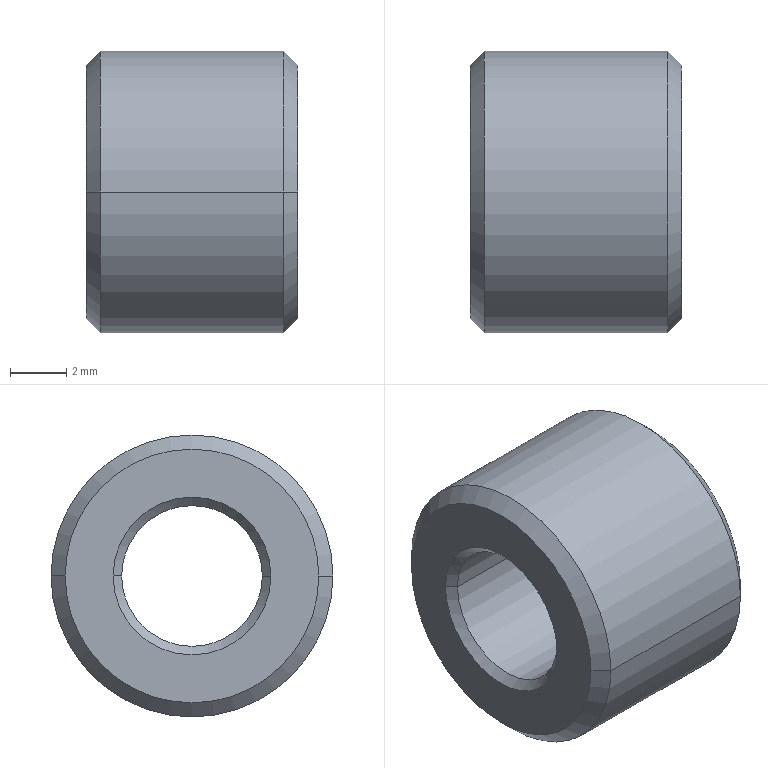Part | STEP file | PRT0008_6_1_2_3_2_1_1 | 1 solid | 14 faces | box 7.5 x 10 x 10 mm | volume 432.724 mm3 | cone 8 | cylinder 4 | plane 2 | commonest cylinder face diameters 5 x2 10 x2
STEP:
#1=CARTESIAN_POINT('',(0.,0.,0.));
#2=DIRECTION('',(0.,0.,1.));
#3=DIRECTION('',(1.,0.,0.));
#4=AXIS2_PLACEMENT_3D('',#1,#2,#3);
#5=CARTESIAN_POINT('',(0.,4.5,0.));
#6=VERTEX_POINT('',#5);
#7=CARTESIAN_POINT('',(0.,0.,4.5));
#8=VERTEX_POINT('',#7);
#9=CARTESIAN_POINT('',(0.,0.,0.));
#10=DIRECTION('',(1.,0.,0.));
#11=DIRECTION('',(0.,1.,0.));
#12=AXIS2_PLACEMENT_3D('',#9,#10,#11);
#13=CIRCLE('',#12,4.5);
#14=EDGE_CURVE('',#6,#8,#13,.T.);
#15=ORIENTED_EDGE('',*,*,#14,.T.);
#16=CARTESIAN_POINT('',(0.,-4.5,0.));
#17=VERTEX_POINT('',#16);
#18=CARTESIAN_POINT('',(0.,0.,0.));
#19=DIRECTION('',(1.,0.,0.));
#20=DIRECTION('',(0.,0.,1.));
#21=AXIS2_PLACEMENT_3D('',#18,#19,#20);
#22=CIRCLE('',#21,4.5);
#23=EDGE_CURVE('',#8,#17,#22,.T.);
#24=ORIENTED_EDGE('',*,*,#23,.T.);
#25=CARTESIAN_POINT('',(0.,0.,-4.5));
#26=VERTEX_POINT('',#25);
#27=CARTESIAN_POINT('',(0.,0.,0.));
#28=DIRECTION('',(1.,0.,0.));
#29=DIRECTION('',(0.,-1.,0.));
#30=AXIS2_PLACEMENT_3D('',#27,#28,#29);
#31=CIRCLE('',#30,4.5);
#32=EDGE_CURVE('',#17,#26,#31,.T.);
#33=ORIENTED_EDGE('',*,*,#32,.T.);
#34=CARTESIAN_POINT('',(0.,0.,0.));
#35=DIRECTION('',(1.,0.,0.));
#36=DIRECTION('',(0.,0.,-1.));
#37=AXIS2_PLACEMENT_3D('',#34,#35,#36);
#38=CIRCLE('',#37,4.5);
#39=EDGE_CURVE('',#26,#6,#38,.T.);
#40=ORIENTED_EDGE('',*,*,#39,.T.);
#41=EDGE_LOOP('',(#15,#24,#33,#40));
#42=FACE_OUTER_BOUND('',#41,.F.);
#43=CARTESIAN_POINT('',(0.,-2.8,0.));
#44=VERTEX_POINT('',#43);
#45=CARTESIAN_POINT('',(0.,0.,2.8));
#46=VERTEX_POINT('',#45);
#47=CARTESIAN_POINT('',(0.,0.,0.));
#48=DIRECTION('',(-1.,0.,0.));
#49=DIRECTION('',(0.,-1.,0.));
#50=AXIS2_PLACEMENT_3D('',#47,#48,#49);
#51=CIRCLE('',#50,2.8);
#52=EDGE_CURVE('',#44,#46,#51,.T.);
#53=ORIENTED_EDGE('',*,*,#52,.T.);
#54=CARTESIAN_POINT('',(0.,2.8,0.));
#55=VERTEX_POINT('',#54);
#56=CARTESIAN_POINT('',(0.,0.,0.));
#57=DIRECTION('',(-1.,0.,0.));
#58=DIRECTION('',(0.,0.,1.));
#59=AXIS2_PLACEMENT_3D('',#56,#57,#58);
#60=CIRCLE('',#59,2.8);
#61=EDGE_CURVE('',#46,#55,#60,.T.);
#62=ORIENTED_EDGE('',*,*,#61,.T.);
#63=CARTESIAN_POINT('',(0.,0.,-2.8));
#64=VERTEX_POINT('',#63);
#65=CARTESIAN_POINT('',(0.,0.,0.));
#66=DIRECTION('',(-1.,0.,0.));
#67=DIRECTION('',(0.,1.,0.));
#68=AXIS2_PLACEMENT_3D('',#65,#66,#67);
#69=CIRCLE('',#68,2.8);
#70=EDGE_CURVE('',#55,#64,#69,.T.);
#71=ORIENTED_EDGE('',*,*,#70,.T.);
#72=CARTESIAN_POINT('',(0.,0.,0.));
#73=DIRECTION('',(-1.,0.,0.));
#74=DIRECTION('',(0.,0.,-1.));
#75=AXIS2_PLACEMENT_3D('',#72,#73,#74);
#76=CIRCLE('',#75,2.8);
#77=EDGE_CURVE('',#64,#44,#76,.T.);
#78=ORIENTED_EDGE('',*,*,#77,.T.);
#79=EDGE_LOOP('',(#53,#62,#71,#78));
#80=FACE_BOUND('',#79,.F.);
#81=CARTESIAN_POINT('',(0.,0.,0.));
#82=DIRECTION('',(1.,0.,0.));
#83=DIRECTION('',(0.,-1.,0.));
#84=AXIS2_PLACEMENT_3D('',#81,#82,#83);
#85=PLANE('',#84);
#86=ADVANCED_FACE('',(#42,#80),#85,.F.);
#87=ORIENTED_EDGE('',*,*,#23,.F.);
#88=ORIENTED_EDGE('',*,*,#14,.F.);
#89=CARTESIAN_POINT('',(0.5,5.,0.));
#90=VERTEX_POINT('',#89);
#91=CARTESIAN_POINT('',(0.,4.5,0.));
#92=DIRECTION('',(0.7071,0.7071,0.));
#93=VECTOR('',#92,0.7071);
#94=LINE('',#91,#93);
#95=EDGE_CURVE('',#6,#90,#94,.T.);
#96=ORIENTED_EDGE('',*,*,#95,.T.);
#97=CARTESIAN_POINT('',(0.5,0.,5.));
#98=VERTEX_POINT('',#97);
#99=CARTESIAN_POINT('',(0.5,0.,0.));
#100=DIRECTION('',(1.,0.,0.));
#101=DIRECTION('',(0.,1.,0.));
#102=AXIS2_PLACEMENT_3D('',#99,#100,#101);
#103=CIRCLE('',#102,5.);
#104=EDGE_CURVE('',#90,#98,#103,.T.);
#105=ORIENTED_EDGE('',*,*,#104,.T.);
#106=CARTESIAN_POINT('',(0.5,-5.,0.));
#107=VERTEX_POINT('',#106);
#108=CARTESIAN_POINT('',(0.5,0.,0.));
#109=DIRECTION('',(1.,0.,0.));
#110=DIRECTION('',(0.,0.,1.));
#111=AXIS2_PLACEMENT_3D('',#108,#109,#110);
#112=CIRCLE('',#111,5.);
#113=EDGE_CURVE('',#98,#107,#112,.T.);
#114=ORIENTED_EDGE('',*,*,#113,.T.);
#115=CARTESIAN_POINT('',(0.,-4.5,0.));
#116=DIRECTION('',(0.7071,-0.7071,0.));
#117=VECTOR('',#116,0.7071);
#118=LINE('',#115,#117);
#119=EDGE_CURVE('',#17,#107,#118,.T.);
#120=ORIENTED_EDGE('',*,*,#119,.F.);
#121=EDGE_LOOP('',(#87,#88,#96,#105,#114,#120));
#122=FACE_OUTER_BOUND('',#121,.F.);
#123=CARTESIAN_POINT('',(0.25,0.,0.));
#124=DIRECTION('',(1.,0.,0.));
#125=DIRECTION('',(0.,0.,-1.));
#126=AXIS2_PLACEMENT_3D('',#123,#124,#125);
#127=CONICAL_SURFACE('',#126,4.75,45.);
#128=ADVANCED_FACE('',(#122),#127,.T.);
#129=ORIENTED_EDGE('',*,*,#39,.F.);
#130=ORIENTED_EDGE('',*,*,#32,.F.);
#131=ORIENTED_EDGE('',*,*,#119,.T.);
#132=CARTESIAN_POINT('',(0.5,0.,-5.));
#133=VERTEX_POINT('',#132);
#134=CARTESIAN_POINT('',(0.5,0.,0.));
#135=DIRECTION('',(1.,0.,0.));
#136=DIRECTION('',(0.,-1.,0.));
#137=AXIS2_PLACEMENT_3D('',#134,#135,#136);
#138=CIRCLE('',#137,5.);
#139=EDGE_CURVE('',#107,#133,#138,.T.);
#140=ORIENTED_EDGE('',*,*,#139,.T.);
#141=CARTESIAN_POINT('',(0.5,0.,0.));
#142=DIRECTION('',(1.,0.,0.));
#143=DIRECTION('',(0.,0.,-1.));
#144=AXIS2_PLACEMENT_3D('',#141,#142,#143);
#145=CIRCLE('',#144,5.);
#146=EDGE_CURVE('',#133,#90,#145,.T.);
#147=ORIENTED_EDGE('',*,*,#146,.T.);
#148=ORIENTED_EDGE('',*,*,#95,.F.);
#149=EDGE_LOOP('',(#129,#130,#131,#140,#147,#148));
#150=FACE_OUTER_BOUND('',#149,.F.);
#151=CARTESIAN_POINT('',(0.25,0.,0.));
#152=DIRECTION('',(1.,0.,0.));
#153=DIRECTION('',(0.,0.,-1.));
#154=AXIS2_PLACEMENT_3D('',#151,#152,#153);
#155=CONICAL_SURFACE('',#154,4.75,45.);
#156=ADVANCED_FACE('',(#150),#155,.T.);
#157=CARTESIAN_POINT('',(7.,0.,-5.));
#158=VERTEX_POINT('',#157);
#159=CARTESIAN_POINT('',(7.,-5.,0.));
#160=VERTEX_POINT('',#159);
#161=CARTESIAN_POINT('',(7.,0.,0.));
#162=DIRECTION('',(-1.,0.,0.));
#163=DIRECTION('',(0.,0.,-1.));
#164=AXIS2_PLACEMENT_3D('',#161,#162,#163);
#165=CIRCLE('',#164,5.);
#166=EDGE_CURVE('',#158,#160,#165,.T.);
#167=ORIENTED_EDGE('',*,*,#166,.F.);
#168=CARTESIAN_POINT('',(7.,5.,0.));
#169=VERTEX_POINT('',#168);
#170=CARTESIAN_POINT('',(7.,0.,0.));
#171=DIRECTION('',(-1.,0.,0.));
#172=DIRECTION('',(0.,1.,0.));
#173=AXIS2_PLACEMENT_3D('',#170,#171,#172);
#174=CIRCLE('',#173,5.);
#175=EDGE_CURVE('',#169,#158,#174,.T.);
#176=ORIENTED_EDGE('',*,*,#175,.F.);
#177=CARTESIAN_POINT('',(0.5,5.,0.));
#178=DIRECTION('',(1.,0.,0.));
#179=VECTOR('',#178,6.5);
#180=LINE('',#177,#179);
#181=EDGE_CURVE('',#90,#169,#180,.T.);
#182=ORIENTED_EDGE('',*,*,#181,.F.);
#183=ORIENTED_EDGE('',*,*,#146,.F.);
#184=ORIENTED_EDGE('',*,*,#139,.F.);
#185=CARTESIAN_POINT('',(0.5,-5.,0.));
#186=DIRECTION('',(1.,0.,0.));
#187=VECTOR('',#186,6.5);
#188=LINE('',#185,#187);
#189=EDGE_CURVE('',#107,#160,#188,.T.);
#190=ORIENTED_EDGE('',*,*,#189,.T.);
#191=EDGE_LOOP('',(#167,#176,#182,#183,#184,#190));
#192=FACE_OUTER_BOUND('',#191,.F.);
#193=CARTESIAN_POINT('',(0.,0.,0.));
#194=DIRECTION('',(1.,0.,0.));
#195=DIRECTION('',(0.,-1.,0.));
#196=AXIS2_PLACEMENT_3D('',#193,#194,#195);
#197=CYLINDRICAL_SURFACE('',#196,5.);
#198=ADVANCED_FACE('',(#192),#197,.T.);
#199=CARTESIAN_POINT('',(7.5,0.,-4.5));
#200=VERTEX_POINT('',#199);
#201=CARTESIAN_POINT('',(7.5,-4.5,0.));
#202=VERTEX_POINT('',#201);
#203=CARTESIAN_POINT('',(7.5,0.,0.));
#204=DIRECTION('',(-1.,0.,0.));
#205=DIRECTION('',(0.,0.,-1.));
#206=AXIS2_PLACEMENT_3D('',#203,#204,#205);
#207=CIRCLE('',#206,4.5);
#208=EDGE_CURVE('',#200,#202,#207,.T.);
#209=ORIENTED_EDGE('',*,*,#208,.F.);
#210=CARTESIAN_POINT('',(7.5,4.5,0.));
#211=VERTEX_POINT('',#210);
#212=CARTESIAN_POINT('',(7.5,0.,0.));
#213=DIRECTION('',(-1.,0.,0.));
#214=DIRECTION('',(0.,1.,0.));
#215=AXIS2_PLACEMENT_3D('',#212,#213,#214);
#216=CIRCLE('',#215,4.5);
#217=EDGE_CURVE('',#211,#200,#216,.T.);
#218=ORIENTED_EDGE('',*,*,#217,.F.);
#219=CARTESIAN_POINT('',(7.5,4.5,0.));
#220=DIRECTION('',(-0.7071,0.7071,0.));
#221=VECTOR('',#220,0.7071);
#222=LINE('',#219,#221);
#223=EDGE_CURVE('',#211,#169,#222,.T.);
#224=ORIENTED_EDGE('',*,*,#223,.T.);
#225=ORIENTED_EDGE('',*,*,#175,.T.);
#226=ORIENTED_EDGE('',*,*,#166,.T.);
#227=CARTESIAN_POINT('',(7.5,-4.5,0.));
#228=DIRECTION('',(-0.7071,-0.7071,0.));
#229=VECTOR('',#228,0.7071);
#230=LINE('',#227,#229);
#231=EDGE_CURVE('',#202,#160,#230,.T.);
#232=ORIENTED_EDGE('',*,*,#231,.F.);
#233=EDGE_LOOP('',(#209,#218,#224,#225,#226,#232));
#234=FACE_OUTER_BOUND('',#233,.F.);
#235=CARTESIAN_POINT('',(7.25,0.,0.));
#236=DIRECTION('',(-1.,0.,0.));
#237=DIRECTION('',(0.,0.,-1.));
#238=AXIS2_PLACEMENT_3D('',#235,#236,#237);
#239=CONICAL_SURFACE('',#238,4.75,45.);
#240=ADVANCED_FACE('',(#234),#239,.T.);
#241=CARTESIAN_POINT('',(7.5,0.,4.5));
#242=VERTEX_POINT('',#241);
#243=CARTESIAN_POINT('',(7.5,0.,0.));
#244=DIRECTION('',(-1.,0.,0.));
#245=DIRECTION('',(0.,-1.,0.));
#246=AXIS2_PLACEMENT_3D('',#243,#244,#245);
#247=CIRCLE('',#246,4.5);
#248=EDGE_CURVE('',#202,#242,#247,.T.);
#249=ORIENTED_EDGE('',*,*,#248,.T.);
#250=CARTESIAN_POINT('',(7.5,0.,0.));
#251=DIRECTION('',(-1.,0.,0.));
#252=DIRECTION('',(0.,0.,1.));
#253=AXIS2_PLACEMENT_3D('',#250,#251,#252);
#254=CIRCLE('',#253,4.5);
#255=EDGE_CURVE('',#242,#211,#254,.T.);
#256=ORIENTED_EDGE('',*,*,#255,.T.);
#257=ORIENTED_EDGE('',*,*,#217,.T.);
#258=ORIENTED_EDGE('',*,*,#208,.T.);
#259=EDGE_LOOP('',(#249,#256,#257,#258));
#260=FACE_OUTER_BOUND('',#259,.F.);
#261=CARTESIAN_POINT('',(7.5,-2.8,0.));
#262=VERTEX_POINT('',#261);
#263=CARTESIAN_POINT('',(7.5,0.,-2.8));
#264=VERTEX_POINT('',#263);
#265=CARTESIAN_POINT('',(7.5,0.,0.));
#266=DIRECTION('',(1.,0.,0.));
#267=DIRECTION('',(0.,-1.,0.));
#268=AXIS2_PLACEMENT_3D('',#265,#266,#267);
#269=CIRCLE('',#268,2.8);
#270=EDGE_CURVE('',#262,#264,#269,.T.);
#271=ORIENTED_EDGE('',*,*,#270,.T.);
#272=CARTESIAN_POINT('',(7.5,2.8,0.));
#273=VERTEX_POINT('',#272);
#274=CARTESIAN_POINT('',(7.5,0.,0.));
#275=DIRECTION('',(1.,0.,0.));
#276=DIRECTION('',(0.,0.,-1.));
#277=AXIS2_PLACEMENT_3D('',#274,#275,#276);
#278=CIRCLE('',#277,2.8);
#279=EDGE_CURVE('',#264,#273,#278,.T.);
#280=ORIENTED_EDGE('',*,*,#279,.T.);
#281=CARTESIAN_POINT('',(7.5,0.,2.8));
#282=VERTEX_POINT('',#281);
#283=CARTESIAN_POINT('',(7.5,0.,0.));
#284=DIRECTION('',(1.,0.,0.));
#285=DIRECTION('',(0.,1.,0.));
#286=AXIS2_PLACEMENT_3D('',#283,#284,#285);
#287=CIRCLE('',#286,2.8);
#288=EDGE_CURVE('',#273,#282,#287,.T.);
#289=ORIENTED_EDGE('',*,*,#288,.T.);
#290=CARTESIAN_POINT('',(7.5,0.,0.));
#291=DIRECTION('',(1.,0.,0.));
#292=DIRECTION('',(0.,0.,1.));
#293=AXIS2_PLACEMENT_3D('',#290,#291,#292);
#294=CIRCLE('',#293,2.8);
#295=EDGE_CURVE('',#282,#262,#294,.T.);
#296=ORIENTED_EDGE('',*,*,#295,.T.);
#297=EDGE_LOOP('',(#271,#280,#289,#296));
#298=FACE_BOUND('',#297,.F.);
#299=CARTESIAN_POINT('',(7.5,0.,0.));
#300=DIRECTION('',(1.,0.,0.));
#301=DIRECTION('',(0.,-1.,0.));
#302=AXIS2_PLACEMENT_3D('',#299,#300,#301);
#303=PLANE('',#302);
#304=ADVANCED_FACE('',(#260,#298),#303,.T.);
#305=ORIENTED_EDGE('',*,*,#255,.F.);
#306=ORIENTED_EDGE('',*,*,#248,.F.);
#307=ORIENTED_EDGE('',*,*,#231,.T.);
#308=CARTESIAN_POINT('',(7.,0.,5.));
#309=VERTEX_POINT('',#308);
#310=CARTESIAN_POINT('',(7.,0.,0.));
#311=DIRECTION('',(-1.,0.,0.));
#312=DIRECTION('',(0.,-1.,0.));
#313=AXIS2_PLACEMENT_3D('',#310,#311,#312);
#314=CIRCLE('',#313,5.);
#315=EDGE_CURVE('',#160,#309,#314,.T.);
#316=ORIENTED_EDGE('',*,*,#315,.T.);
#317=CARTESIAN_POINT('',(7.,0.,0.));
#318=DIRECTION('',(-1.,0.,0.));
#319=DIRECTION('',(0.,0.,1.));
#320=AXIS2_PLACEMENT_3D('',#317,#318,#319);
#321=CIRCLE('',#320,5.);
#322=EDGE_CURVE('',#309,#169,#321,.T.);
#323=ORIENTED_EDGE('',*,*,#322,.T.);
#324=ORIENTED_EDGE('',*,*,#223,.F.);
#325=EDGE_LOOP('',(#305,#306,#307,#316,#323,#324));
#326=FACE_OUTER_BOUND('',#325,.F.);
#327=CARTESIAN_POINT('',(7.25,0.,0.));
#328=DIRECTION('',(-1.,0.,0.));
#329=DIRECTION('',(0.,0.,-1.));
#330=AXIS2_PLACEMENT_3D('',#327,#328,#329);
#331=CONICAL_SURFACE('',#330,4.75,45.);
#332=ADVANCED_FACE('',(#326),#331,.T.);
#333=ORIENTED_EDGE('',*,*,#322,.F.);
#334=ORIENTED_EDGE('',*,*,#315,.F.);
#335=ORIENTED_EDGE('',*,*,#189,.F.);
#336=ORIENTED_EDGE('',*,*,#113,.F.);
#337=ORIENTED_EDGE('',*,*,#104,.F.);
#338=ORIENTED_EDGE('',*,*,#181,.T.);
#339=EDGE_LOOP('',(#333,#334,#335,#336,#337,#338));
#340=FACE_OUTER_BOUND('',#339,.F.);
#341=CARTESIAN_POINT('',(0.,0.,0.));
#342=DIRECTION('',(1.,0.,0.));
#343=DIRECTION('',(0.,-1.,0.));
#344=AXIS2_PLACEMENT_3D('',#341,#342,#343);
#345=CYLINDRICAL_SURFACE('',#344,5.);
#346=ADVANCED_FACE('',(#340),#345,.T.);
#347=ORIENTED_EDGE('',*,*,#279,.F.);
#348=ORIENTED_EDGE('',*,*,#270,.F.);
#349=CARTESIAN_POINT('',(7.2,-2.5,0.));
#350=VERTEX_POINT('',#349);
#351=CARTESIAN_POINT('',(7.5,-2.8,0.));
#352=DIRECTION('',(-0.7071,0.7071,0.));
#353=VECTOR('',#352,0.4243);
#354=LINE('',#351,#353);
#355=EDGE_CURVE('',#262,#350,#354,.T.);
#356=ORIENTED_EDGE('',*,*,#355,.T.);
#357=CARTESIAN_POINT('',(7.2,0.,-2.5));
#358=VERTEX_POINT('',#357);
#359=CARTESIAN_POINT('',(7.2,0.,0.));
#360=DIRECTION('',(1.,0.,0.));
#361=DIRECTION('',(0.,-1.,0.));
#362=AXIS2_PLACEMENT_3D('',#359,#360,#361);
#363=CIRCLE('',#362,2.5);
#364=EDGE_CURVE('',#350,#358,#363,.T.);
#365=ORIENTED_EDGE('',*,*,#364,.T.);
#366=CARTESIAN_POINT('',(7.2,2.5,0.000000001));
#367=VERTEX_POINT('',#366);
#368=CARTESIAN_POINT('',(7.2,0.,0.));
#369=DIRECTION('',(1.,0.,0.));
#370=DIRECTION('',(0.,0.,-1.));
#371=AXIS2_PLACEMENT_3D('',#368,#369,#370);
#372=CIRCLE('',#371,2.5);
#373=EDGE_CURVE('',#358,#367,#372,.T.);
#374=ORIENTED_EDGE('',*,*,#373,.T.);
#375=CARTESIAN_POINT('',(7.5,2.8,0.000000001));
#376=DIRECTION('',(-0.7071,-0.7071,0.000000001));
#377=VECTOR('',#376,0.4243);
#378=LINE('',#375,#377);
#379=EDGE_CURVE('',#273,#367,#378,.T.);
#380=ORIENTED_EDGE('',*,*,#379,.F.);
#381=EDGE_LOOP('',(#347,#348,#356,#365,#374,#380));
#382=FACE_OUTER_BOUND('',#381,.F.);
#383=CARTESIAN_POINT('',(7.35,0.,0.));
#384=DIRECTION('',(1.,0.,0.));
#385=DIRECTION('',(0.,0.,-1.));
#386=AXIS2_PLACEMENT_3D('',#383,#384,#385);
#387=CONICAL_SURFACE('',#386,2.65,45.);
#388=ADVANCED_FACE('',(#382),#387,.F.);
#389=ORIENTED_EDGE('',*,*,#295,.F.);
#390=ORIENTED_EDGE('',*,*,#288,.F.);
#391=ORIENTED_EDGE('',*,*,#379,.T.);
#392=CARTESIAN_POINT('',(7.2,0.,2.5));
#393=VERTEX_POINT('',#392);
#394=CARTESIAN_POINT('',(7.2,0.,0.));
#395=DIRECTION('',(1.,0.,0.));
#396=DIRECTION('',(0.,1.,0.));
#397=AXIS2_PLACEMENT_3D('',#394,#395,#396);
#398=CIRCLE('',#397,2.5);
#399=EDGE_CURVE('',#367,#393,#398,.T.);
#400=ORIENTED_EDGE('',*,*,#399,.T.);
#401=CARTESIAN_POINT('',(7.2,0.,0.));
#402=DIRECTION('',(1.,0.,0.));
#403=DIRECTION('',(0.,0.,1.));
#404=AXIS2_PLACEMENT_3D('',#401,#402,#403);
#405=CIRCLE('',#404,2.5);
#406=EDGE_CURVE('',#393,#350,#405,.T.);
#407=ORIENTED_EDGE('',*,*,#406,.T.);
#408=ORIENTED_EDGE('',*,*,#355,.F.);
#409=EDGE_LOOP('',(#389,#390,#391,#400,#407,#408));
#410=FACE_OUTER_BOUND('',#409,.F.);
#411=CARTESIAN_POINT('',(7.35,0.,0.));
#412=DIRECTION('',(1.,0.,0.));
#413=DIRECTION('',(0.,0.,-1.));
#414=AXIS2_PLACEMENT_3D('',#411,#412,#413);
#415=CONICAL_SURFACE('',#414,2.65,45.);
#416=ADVANCED_FACE('',(#410),#415,.F.);
#417=ORIENTED_EDGE('',*,*,#406,.F.);
#418=ORIENTED_EDGE('',*,*,#399,.F.);
#419=CARTESIAN_POINT('',(0.3,2.5,0.000000001));
#420=VERTEX_POINT('',#419);
#421=CARTESIAN_POINT('',(0.3,2.5,0.000000001));
#422=DIRECTION('',(1.,0.,0.));
#423=VECTOR('',#422,6.9);
#424=LINE('',#421,#423);
#425=EDGE_CURVE('',#420,#367,#424,.T.);
#426=ORIENTED_EDGE('',*,*,#425,.F.);
#427=CARTESIAN_POINT('',(0.3,0.,2.5));
#428=VERTEX_POINT('',#427);
#429=CARTESIAN_POINT('',(0.3,0.,0.));
#430=DIRECTION('',(-1.,0.,0.));
#431=DIRECTION('',(0.,0.,1.));
#432=AXIS2_PLACEMENT_3D('',#429,#430,#431);
#433=CIRCLE('',#432,2.5);
#434=EDGE_CURVE('',#428,#420,#433,.T.);
#435=ORIENTED_EDGE('',*,*,#434,.F.);
#436=CARTESIAN_POINT('',(0.3,-2.5,0.));
#437=VERTEX_POINT('',#436);
#438=CARTESIAN_POINT('',(0.3,0.,0.));
#439=DIRECTION('',(-1.,0.,0.));
#440=DIRECTION('',(0.,-1.,0.));
#441=AXIS2_PLACEMENT_3D('',#438,#439,#440);
#442=CIRCLE('',#441,2.5);
#443=EDGE_CURVE('',#437,#428,#442,.T.);
#444=ORIENTED_EDGE('',*,*,#443,.F.);
#445=CARTESIAN_POINT('',(0.3,-2.5,0.));
#446=DIRECTION('',(1.,0.,0.));
#447=VECTOR('',#446,6.9);
#448=LINE('',#445,#447);
#449=EDGE_CURVE('',#437,#350,#448,.T.);
#450=ORIENTED_EDGE('',*,*,#449,.T.);
#451=EDGE_LOOP('',(#417,#418,#426,#435,#444,#450));
#452=FACE_OUTER_BOUND('',#451,.F.);
#453=CARTESIAN_POINT('',(0.,0.,0.));
#454=DIRECTION('',(1.,0.,0.));
#455=DIRECTION('',(0.,-1.,0.));
#456=AXIS2_PLACEMENT_3D('',#453,#454,#455);
#457=CYLINDRICAL_SURFACE('',#456,2.5);
#458=ADVANCED_FACE('',(#452),#457,.F.);
#459=ORIENTED_EDGE('',*,*,#373,.F.);
#460=ORIENTED_EDGE('',*,*,#364,.F.);
#461=ORIENTED_EDGE('',*,*,#449,.F.);
#462=CARTESIAN_POINT('',(0.3,0.,-2.5));
#463=VERTEX_POINT('',#462);
#464=CARTESIAN_POINT('',(0.3,0.,0.));
#465=DIRECTION('',(-1.,0.,0.));
#466=DIRECTION('',(0.,0.,-1.));
#467=AXIS2_PLACEMENT_3D('',#464,#465,#466);
#468=CIRCLE('',#467,2.5);
#469=EDGE_CURVE('',#463,#437,#468,.T.);
#470=ORIENTED_EDGE('',*,*,#469,.F.);
#471=CARTESIAN_POINT('',(0.3,0.,0.));
#472=DIRECTION('',(-1.,0.,0.));
#473=DIRECTION('',(0.,1.,0.));
#474=AXIS2_PLACEMENT_3D('',#471,#472,#473);
#475=CIRCLE('',#474,2.5);
#476=EDGE_CURVE('',#420,#463,#475,.T.);
#477=ORIENTED_EDGE('',*,*,#476,.F.);
#478=ORIENTED_EDGE('',*,*,#425,.T.);
#479=EDGE_LOOP('',(#459,#460,#461,#470,#477,#478));
#480=FACE_OUTER_BOUND('',#479,.F.);
#481=CARTESIAN_POINT('',(0.,0.,0.));
#482=DIRECTION('',(1.,0.,0.));
#483=DIRECTION('',(0.,-1.,0.));
#484=AXIS2_PLACEMENT_3D('',#481,#482,#483);
#485=CYLINDRICAL_SURFACE('',#484,2.5);
#486=ADVANCED_FACE('',(#480),#485,.F.);
#487=ORIENTED_EDGE('',*,*,#77,.F.);
#488=ORIENTED_EDGE('',*,*,#70,.F.);
#489=CARTESIAN_POINT('',(0.,2.8,0.000000001));
#490=DIRECTION('',(0.7071,-0.7071,0.000000001));
#491=VECTOR('',#490,0.4243);
#492=LINE('',#489,#491);
#493=EDGE_CURVE('',#55,#420,#492,.T.);
#494=ORIENTED_EDGE('',*,*,#493,.T.);
#495=ORIENTED_EDGE('',*,*,#476,.T.);
#496=ORIENTED_EDGE('',*,*,#469,.T.);
#497=CARTESIAN_POINT('',(0.,-2.8,0.));
#498=DIRECTION('',(0.7071,0.7071,0.));
#499=VECTOR('',#498,0.4243);
#500=LINE('',#497,#499);
#501=EDGE_CURVE('',#44,#437,#500,.T.);
#502=ORIENTED_EDGE('',*,*,#501,.F.);
#503=EDGE_LOOP('',(#487,#488,#494,#495,#496,#502));
#504=FACE_OUTER_BOUND('',#503,.F.);
#505=CARTESIAN_POINT('',(0.15,0.,0.));
#506=DIRECTION('',(-1.,0.,0.));
#507=DIRECTION('',(0.,0.,-1.));
#508=AXIS2_PLACEMENT_3D('',#505,#506,#507);
#509=CONICAL_SURFACE('',#508,2.65,45.);
#510=ADVANCED_FACE('',(#504),#509,.F.);
#511=ORIENTED_EDGE('',*,*,#61,.F.);
#512=ORIENTED_EDGE('',*,*,#52,.F.);
#513=ORIENTED_EDGE('',*,*,#501,.T.);
#514=ORIENTED_EDGE('',*,*,#443,.T.);
#515=ORIENTED_EDGE('',*,*,#434,.T.);
#516=ORIENTED_EDGE('',*,*,#493,.F.);
#517=EDGE_LOOP('',(#511,#512,#513,#514,#515,#516));
#518=FACE_OUTER_BOUND('',#517,.F.);
#519=CARTESIAN_POINT('',(0.15,0.,0.));
#520=DIRECTION('',(-1.,0.,0.));
#521=DIRECTION('',(0.,0.,-1.));
#522=AXIS2_PLACEMENT_3D('',#519,#520,#521);
#523=CONICAL_SURFACE('',#522,2.65,45.);
#524=ADVANCED_FACE('',(#518),#523,.F.);
#525=CLOSED_SHELL('',(#86,#128,#156,#198,#240,#304,#332,#346,#388,#416,#458,#486,#510,#524));
#526=MANIFOLD_SOLID_BREP('',#525);
#527=(LENGTH_UNIT()NAMED_UNIT(*)SI_UNIT(.MILLI.,.METRE.));
#528=UNCERTAINTY_MEASURE_WITH_UNIT(LENGTH_MEASURE(0.001601),#527,'','');
#529=(NAMED_UNIT(*)PLANE_ANGLE_UNIT()SI_UNIT($,.RADIAN.));
#530=PLANE_ANGLE_MEASURE_WITH_UNIT(PLANE_ANGLE_MEASURE(0.01745),#529);
#531=(CONVERSION_BASED_UNIT('DEGREE',#530)NAMED_UNIT(*)PLANE_ANGLE_UNIT());
#532=(NAMED_UNIT(*)SI_UNIT($,.STERADIAN.)SOLID_ANGLE_UNIT());
#533=(GEOMETRIC_REPRESENTATION_CONTEXT(3)GLOBAL_UNCERTAINTY_ASSIGNED_CONTEXT((#528))GLOBAL_UNIT_ASSIGNED_CONTEXT((#527,#531,#532))REPRESENTATION_CONTEXT('',''));
#534=ADVANCED_BREP_SHAPE_REPRESENTATION('',(#4,#526),#533);